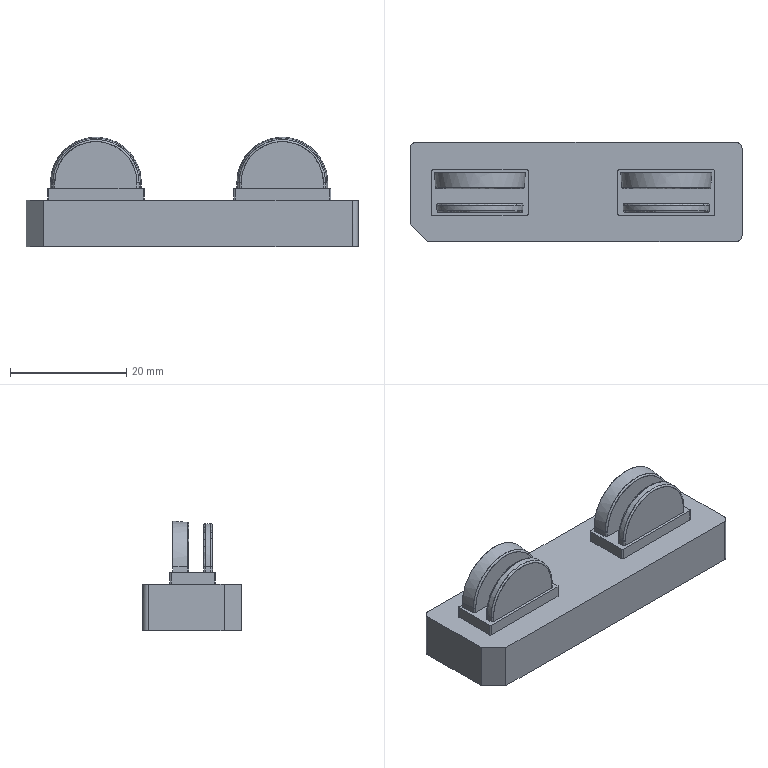CAM job | PowerMill | 3-axis milling, other | part box 57 x 17 x 18.807 mm
Tools:
number,name,type,diameter,tip_radius,length,cutting_length,overhang,flutes,holder,toolpaths_using
1,D10C,end_mill,10.0,0.0,60.0,,30.0,1,D42L35,1
2,D4C,end_mill,4.0,0.0,30.0,,15.0,1,D42L35,1
1,D10C_1_1_1,end_mill,10.0,0.0,60.0,,19.24,1,D42L35,3
2,D4C_1_1,end_mill,4.0,0.0,30.0,,11.0,1,D42L35,2
28,D2C_1_1,end_mill,2.0,0.0,8.72,,9.04,1,D42L35,1
3,D10_1_1_1,end_mill,10.0,0.0,60.0,,18.96,1,D42L35,3
4,R1_1_1,ball_nosed,2.0,1.0,4.36,,8.88,1,D42L35,1
12,D2_1_1,end_mill,2.0,0.0,9.16,,9.16,1,D42L35,1
13,Text_D4_1_1,taper_spherical,4.0,0.3,60.0,,11.08,1,D42L35,1
Operations:
program,toolpath,strategy,tool,tool_number,tool_diameter,tip_radius,flutes,spindle_rpm,feed_cut,surface_speed_m_min_computed,feed_per_tooth_computed,tolerance,thickness,stepover,stepdown,cut_length,cut_time_min,total_time_min,workplane
18-S-2-F,精公开粗01-扫面平行-D10C,raster_area_clear,D10C_1_1_1,1,10.0,0.0,1.0,8000.0,10000.0,251.33,1.25,0.03,0.28,6.0,1.0,335.36,0.034,0.0395,
18-S-2-F,精公开粗01-外形偏置-D10C,offset_area_clear,D10C_1_1_1,1,10.0,0.0,1.0,8000.0,10000.0,251.33,1.25,0.03,0.28,6.0,1.0,9276.079,0.928,0.9964,
18-S-2-F,精公开粗01-基准台等高-D10C,constantz,D10C_1_1_1,1,10.0,0.0,1.0,8000.0,10000.0,251.33,1.25,0.03,0.07,5.0,0.4,3889.064,0.389,0.3996,
18-S-2-F,精公再粗02-外形偏置-D4C,offset_area_clear,D4C_1_1,2,4.0,0.0,1.0,18000.0,6000.0,226.19,0.3333,0.03,0.0,2.0,1.0,6185.632,1.031,1.095,
18-S-2-F,精公再粗02-平行中光-D4C,raster,D4C_1_1,2,4.0,0.0,1.0,18000.0,6000.0,226.19,0.3333,0.03,0.0,0.2,1.0,2624.686,0.437,0.4586,
18-S-2-F,精公再粗03-外形偏置-D2C,offset_area_clear,D2C_1_1,28,2.0,0.0,1.0,18000.0,4000.0,113.1,0.2222,0.03,0.0,1.1,1.0,4748.286,1.187,1.513,
18-S-2-F,精公基准台01-基准面偏置-D10,offset_area_clear,D10_1_1_1,3,10.0,0.0,1.0,8500.0,600.0,267.04,0.0706,0.005,0.38,5.0,1.0,183.099,0.305,0.3451,
18-S-2-F,精公基准台01-外形侧光-D10,profile_area_clear,D10_1_1_1,3,10.0,0.0,1.0,8500.0,600.0,267.04,0.0706,0.005,-0.07,0.08,1.0,318.926,0.532,0.5722,
18-S-2-F,精公基准台01-基准台侧光-D10,profile_area_clear,D10_1_1_1,3,10.0,0.0,1.0,8500.0,600.0,267.04,0.0706,0.005,0.0,0.08,1.0,353.233,0.589,0.6538,
18-S-2-F,精公精光01-浅滩和陡峭-R1,inter_constz,R1_1_1,4,2.0,1.0,1.0,18000.0,2000.0,113.1,0.1111,0.005,-0.075,0.03,1.0,15493.934,7.747,8.473,
18-S-2-F,精公精光02-等高-D2,constantz,D2_1_1,12,2.0,0.0,1.0,18000.0,1500.0,113.1,0.0833,0.005,-0.075,5.0,0.03,39672.02,26.448,26.487,
18-S-2-F,精公刻字01-刻字-Text_D4,pattern,Text_D4_1_1,13,4.0,0.3,1.0,15000.0,1000.0,188.5,0.0667,0.005,0.0,5.0,1.0,38.916,0.039,0.0545,
,精公开粗01-外形偏置-D10C_Reference,offset_area_clear,D10C,1,10.0,0.0,1.0,8000.0,10000.0,251.33,1.25,0.03,0.28,6.0,1.0,18561.265,1.856,1.99,
,精公再粗02-外形偏置-D4C_Reference,offset_area_clear,D4C,2,4.0,0.0,1.0,18000.0,6000.0,226.19,0.3333,0.03,0.0,2.0,1.0,11970.217,1.995,2.091,